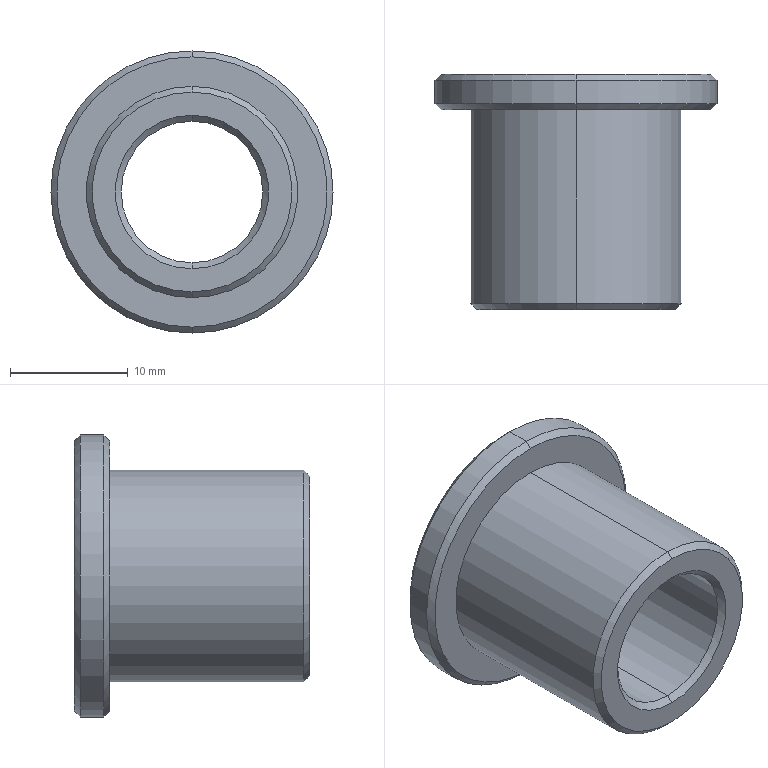Part | SolidWorks | features BaseBody 1 | 1 solid | 19 faces | box 24 x 20 x 24 mm | volume 3357 mm3 | cone 10 | cylinder 6 | plane 3 | commonest cylinder face diameters 12.05 x2 17.98 x2 24 x2
STEP:
#1=CARTESIAN_POINT('',(375.1,-76.45,75.025));
#2=VERTEX_POINT('',#1);
#3=CARTESIAN_POINT('',(375.1,-76.45,62.975));
#4=VERTEX_POINT('',#3);
#5=CARTESIAN_POINT('',(375.1,-76.45,69.));
#6=DIRECTION('',(0.,-1.,0.));
#7=DIRECTION('',(0.,0.,1.));
#8=AXIS2_PLACEMENT_3D('',#5,#6,#7);
#9=CIRCLE('',#8,6.025);
#10=EDGE_CURVE('',#2,#4,#9,.T.);
#11=ORIENTED_EDGE('',*,*,#10,.T.);
#12=CARTESIAN_POINT('',(375.1,-75.95,62.475));
#13=VERTEX_POINT('',#12);
#14=CARTESIAN_POINT('',(375.1,-76.2,62.725));
#15=DIRECTION('',(0.,0.7071,-0.7071));
#16=VECTOR('',#15,1000.);
#17=LINE('',#14,#16);
#18=EDGE_CURVE('',#4,#13,#17,.T.);
#19=ORIENTED_EDGE('',*,*,#18,.T.);
#20=CARTESIAN_POINT('',(375.1,-75.95,75.525));
#21=VERTEX_POINT('',#20);
#22=CARTESIAN_POINT('',(375.1,-75.95,69.));
#23=DIRECTION('',(0.,-1.,0.));
#24=DIRECTION('',(0.,0.,1.));
#25=AXIS2_PLACEMENT_3D('',#22,#23,#24);
#26=CIRCLE('',#25,6.525);
#27=EDGE_CURVE('',#21,#13,#26,.T.);
#28=ORIENTED_EDGE('',*,*,#27,.F.);
#29=CARTESIAN_POINT('',(375.1,-76.2,75.275));
#30=DIRECTION('',(0.,0.7071,0.7071));
#31=VECTOR('',#30,1000.);
#32=LINE('',#29,#31);
#33=EDGE_CURVE('',#2,#21,#32,.T.);
#34=ORIENTED_EDGE('',*,*,#33,.F.);
#35=EDGE_LOOP('',(#11,#19,#28,#34));
#36=FACE_OUTER_BOUND('',#35,.T.);
#37=CARTESIAN_POINT('',(375.1,-76.2,69.));
#38=DIRECTION('',(0.,1.,0.));
#39=DIRECTION('',(0.,0.,1.));
#40=AXIS2_PLACEMENT_3D('',#37,#38,#39);
#41=CONICAL_SURFACE('',#40,6.275,0.7854);
#42=ADVANCED_FACE('',(#36),#41,.F.);
#43=CARTESIAN_POINT('',(375.1,-95.45,62.975));
#44=VERTEX_POINT('',#43);
#45=CARTESIAN_POINT('',(375.1,-95.45,75.025));
#46=VERTEX_POINT('',#45);
#47=CARTESIAN_POINT('',(375.1,-95.45,69.));
#48=DIRECTION('',(0.,1.,0.));
#49=DIRECTION('',(0.,0.,-1.));
#50=AXIS2_PLACEMENT_3D('',#47,#48,#49);
#51=CIRCLE('',#50,6.025);
#52=EDGE_CURVE('',#44,#46,#51,.T.);
#53=ORIENTED_EDGE('',*,*,#52,.F.);
#54=CARTESIAN_POINT('',(375.1,-78.95,62.975));
#55=DIRECTION('',(0.,1.,0.));
#56=VECTOR('',#55,1000.);
#57=LINE('',#54,#56);
#58=EDGE_CURVE('',#44,#4,#57,.T.);
#59=ORIENTED_EDGE('',*,*,#58,.T.);
#60=ORIENTED_EDGE('',*,*,#10,.F.);
#61=CARTESIAN_POINT('',(375.1,-78.95,75.025));
#62=DIRECTION('',(0.,1.,0.));
#63=VECTOR('',#62,1000.);
#64=LINE('',#61,#63);
#65=EDGE_CURVE('',#46,#2,#64,.T.);
#66=ORIENTED_EDGE('',*,*,#65,.F.);
#67=EDGE_LOOP('',(#53,#59,#60,#66));
#68=FACE_OUTER_BOUND('',#67,.T.);
#69=CARTESIAN_POINT('',(375.1,-78.95,69.));
#70=DIRECTION('',(0.,1.,0.));
#71=DIRECTION('',(0.,0.,1.));
#72=AXIS2_PLACEMENT_3D('',#69,#70,#71);
#73=CYLINDRICAL_SURFACE('',#72,6.025);
#74=ADVANCED_FACE('',(#68),#73,.F.);
#75=ORIENTED_EDGE('',*,*,#52,.T.);
#76=CARTESIAN_POINT('',(375.1,-95.95,75.525));
#77=VERTEX_POINT('',#76);
#78=CARTESIAN_POINT('',(375.1,-95.7,75.275));
#79=DIRECTION('',(0.,-0.7071,0.7071));
#80=VECTOR('',#79,1000.);
#81=LINE('',#78,#80);
#82=EDGE_CURVE('',#46,#77,#81,.T.);
#83=ORIENTED_EDGE('',*,*,#82,.T.);
#84=CARTESIAN_POINT('',(375.1,-95.95,62.475));
#85=VERTEX_POINT('',#84);
#86=CARTESIAN_POINT('',(375.1,-95.95,69.));
#87=DIRECTION('',(0.,1.,0.));
#88=DIRECTION('',(0.,0.,-1.));
#89=AXIS2_PLACEMENT_3D('',#86,#87,#88);
#90=CIRCLE('',#89,6.525);
#91=EDGE_CURVE('',#85,#77,#90,.T.);
#92=ORIENTED_EDGE('',*,*,#91,.F.);
#93=CARTESIAN_POINT('',(375.1,-95.7,62.725));
#94=DIRECTION('',(0.,-0.7071,-0.7071));
#95=VECTOR('',#94,1000.);
#96=LINE('',#93,#95);
#97=EDGE_CURVE('',#44,#85,#96,.T.);
#98=ORIENTED_EDGE('',*,*,#97,.F.);
#99=EDGE_LOOP('',(#75,#83,#92,#98));
#100=FACE_OUTER_BOUND('',#99,.T.);
#101=CARTESIAN_POINT('',(375.1,-95.7,69.));
#102=DIRECTION('',(0.,-1.,0.));
#103=DIRECTION('',(0.,0.,-1.));
#104=AXIS2_PLACEMENT_3D('',#101,#102,#103);
#105=CONICAL_SURFACE('',#104,6.275,0.7854);
#106=ADVANCED_FACE('',(#100),#105,.F.);
#107=CARTESIAN_POINT('',(375.1,-75.95,80.5));
#108=VERTEX_POINT('',#107);
#109=CARTESIAN_POINT('',(375.1,-75.95,57.5));
#110=VERTEX_POINT('',#109);
#111=CARTESIAN_POINT('',(375.1,-75.95,69.));
#112=DIRECTION('',(0.,1.,0.));
#113=DIRECTION('',(0.,0.,-1.));
#114=AXIS2_PLACEMENT_3D('',#111,#112,#113);
#115=CIRCLE('',#114,11.5);
#116=EDGE_CURVE('',#108,#110,#115,.T.);
#117=ORIENTED_EDGE('',*,*,#116,.F.);
#118=CARTESIAN_POINT('',(375.1,-76.45,81.));
#119=VERTEX_POINT('',#118);
#120=CARTESIAN_POINT('',(375.1,-76.2,80.75));
#121=DIRECTION('',(0.,-0.7071,0.7071));
#122=VECTOR('',#121,1000.);
#123=LINE('',#120,#122);
#124=EDGE_CURVE('',#108,#119,#123,.T.);
#125=ORIENTED_EDGE('',*,*,#124,.T.);
#126=CARTESIAN_POINT('',(375.1,-76.45,57.));
#127=VERTEX_POINT('',#126);
#128=CARTESIAN_POINT('',(375.1,-76.45,69.));
#129=DIRECTION('',(0.,1.,0.));
#130=DIRECTION('',(0.,0.,-1.));
#131=AXIS2_PLACEMENT_3D('',#128,#129,#130);
#132=CIRCLE('',#131,12.);
#133=EDGE_CURVE('',#119,#127,#132,.T.);
#134=ORIENTED_EDGE('',*,*,#133,.T.);
#135=CARTESIAN_POINT('',(375.1,-76.2,57.25));
#136=DIRECTION('',(0.,-0.7071,-0.7071));
#137=VECTOR('',#136,1000.);
#138=LINE('',#135,#137);
#139=EDGE_CURVE('',#110,#127,#138,.T.);
#140=ORIENTED_EDGE('',*,*,#139,.F.);
#141=EDGE_LOOP('',(#117,#125,#134,#140));
#142=FACE_OUTER_BOUND('',#141,.T.);
#143=CARTESIAN_POINT('',(375.1,-76.2,69.));
#144=DIRECTION('',(0.,-1.,0.));
#145=DIRECTION('',(0.,0.,-1.));
#146=AXIS2_PLACEMENT_3D('',#143,#144,#145);
#147=CONICAL_SURFACE('',#146,11.75,0.7854);
#148=ADVANCED_FACE('',(#142),#147,.T.);
#149=CARTESIAN_POINT('',(375.1,-78.45,57.));
#150=VERTEX_POINT('',#149);
#151=CARTESIAN_POINT('',(375.1,-78.45,81.));
#152=VERTEX_POINT('',#151);
#153=CARTESIAN_POINT('',(375.1,-78.45,69.));
#154=DIRECTION('',(0.,-1.,0.));
#155=DIRECTION('',(0.,0.,-1.));
#156=AXIS2_PLACEMENT_3D('',#153,#154,#155);
#157=CIRCLE('',#156,12.);
#158=EDGE_CURVE('',#150,#152,#157,.T.);
#159=ORIENTED_EDGE('',*,*,#158,.F.);
#160=CARTESIAN_POINT('',(375.1,-78.95,57.));
#161=DIRECTION('',(0.,1.,0.));
#162=VECTOR('',#161,1000.);
#163=LINE('',#160,#162);
#164=EDGE_CURVE('',#150,#127,#163,.T.);
#165=ORIENTED_EDGE('',*,*,#164,.T.);
#166=ORIENTED_EDGE('',*,*,#133,.F.);
#167=CARTESIAN_POINT('',(375.1,-78.95,81.));
#168=DIRECTION('',(0.,1.,0.));
#169=VECTOR('',#168,1000.);
#170=LINE('',#167,#169);
#171=EDGE_CURVE('',#152,#119,#170,.T.);
#172=ORIENTED_EDGE('',*,*,#171,.F.);
#173=EDGE_LOOP('',(#159,#165,#166,#172));
#174=FACE_OUTER_BOUND('',#173,.T.);
#175=CARTESIAN_POINT('',(375.1,-78.95,69.));
#176=DIRECTION('',(0.,1.,0.));
#177=DIRECTION('',(0.,0.,1.));
#178=AXIS2_PLACEMENT_3D('',#175,#176,#177);
#179=CYLINDRICAL_SURFACE('',#178,12.);
#180=ADVANCED_FACE('',(#174),#179,.T.);
#181=CARTESIAN_POINT('',(375.1,-78.95,57.5));
#182=VERTEX_POINT('',#181);
#183=CARTESIAN_POINT('',(375.1,-78.95,80.5));
#184=VERTEX_POINT('',#183);
#185=CARTESIAN_POINT('',(375.1,-78.95,69.));
#186=DIRECTION('',(0.,-1.,0.));
#187=DIRECTION('',(0.,0.,1.));
#188=AXIS2_PLACEMENT_3D('',#185,#186,#187);
#189=CIRCLE('',#188,11.5);
#190=EDGE_CURVE('',#182,#184,#189,.T.);
#191=ORIENTED_EDGE('',*,*,#190,.F.);
#192=CARTESIAN_POINT('',(375.1,-78.7,57.25));
#193=DIRECTION('',(0.,0.7071,-0.7071));
#194=VECTOR('',#193,1000.);
#195=LINE('',#192,#194);
#196=EDGE_CURVE('',#182,#150,#195,.T.);
#197=ORIENTED_EDGE('',*,*,#196,.T.);
#198=ORIENTED_EDGE('',*,*,#158,.T.);
#199=CARTESIAN_POINT('',(375.1,-78.7,80.75));
#200=DIRECTION('',(0.,0.7071,0.7071));
#201=VECTOR('',#200,1000.);
#202=LINE('',#199,#201);
#203=EDGE_CURVE('',#184,#152,#202,.T.);
#204=ORIENTED_EDGE('',*,*,#203,.F.);
#205=EDGE_LOOP('',(#191,#197,#198,#204));
#206=FACE_OUTER_BOUND('',#205,.T.);
#207=CARTESIAN_POINT('',(375.1,-78.7,69.));
#208=DIRECTION('',(0.,1.,0.));
#209=DIRECTION('',(0.,0.,1.));
#210=AXIS2_PLACEMENT_3D('',#207,#208,#209);
#211=CONICAL_SURFACE('',#210,11.75,0.7854);
#212=ADVANCED_FACE('',(#206),#211,.T.);
#213=CARTESIAN_POINT('',(375.1,-95.45,60.01));
#214=VERTEX_POINT('',#213);
#215=CARTESIAN_POINT('',(375.1,-95.45,77.99));
#216=VERTEX_POINT('',#215);
#217=CARTESIAN_POINT('',(375.1,-95.45,69.));
#218=DIRECTION('',(0.,-1.,0.));
#219=DIRECTION('',(0.,0.,-1.));
#220=AXIS2_PLACEMENT_3D('',#217,#218,#219);
#221=CIRCLE('',#220,8.99);
#222=EDGE_CURVE('',#214,#216,#221,.T.);
#223=ORIENTED_EDGE('',*,*,#222,.F.);
#224=CARTESIAN_POINT('',(375.1,-78.95,60.01));
#225=VERTEX_POINT('',#224);
#226=CARTESIAN_POINT('',(375.1,-95.95,60.01));
#227=DIRECTION('',(0.,1.,0.));
#228=VECTOR('',#227,1000.);
#229=LINE('',#226,#228);
#230=EDGE_CURVE('',#214,#225,#229,.T.);
#231=ORIENTED_EDGE('',*,*,#230,.T.);
#232=CARTESIAN_POINT('',(375.1,-78.95,77.99));
#233=VERTEX_POINT('',#232);
#234=CARTESIAN_POINT('',(375.1,-78.95,69.));
#235=DIRECTION('',(0.,1.,0.));
#236=DIRECTION('',(0.,0.,-1.));
#237=AXIS2_PLACEMENT_3D('',#234,#235,#236);
#238=CIRCLE('',#237,8.99);
#239=EDGE_CURVE('',#233,#225,#238,.T.);
#240=ORIENTED_EDGE('',*,*,#239,.F.);
#241=CARTESIAN_POINT('',(375.1,-95.95,77.99));
#242=DIRECTION('',(0.,1.,0.));
#243=VECTOR('',#242,1000.);
#244=LINE('',#241,#243);
#245=EDGE_CURVE('',#216,#233,#244,.T.);
#246=ORIENTED_EDGE('',*,*,#245,.F.);
#247=EDGE_LOOP('',(#223,#231,#240,#246));
#248=FACE_OUTER_BOUND('',#247,.T.);
#249=CARTESIAN_POINT('',(375.1,-95.95,69.));
#250=DIRECTION('',(0.,1.,0.));
#251=DIRECTION('',(0.,0.,1.));
#252=AXIS2_PLACEMENT_3D('',#249,#250,#251);
#253=CYLINDRICAL_SURFACE('',#252,8.99);
#254=ADVANCED_FACE('',(#248),#253,.T.);
#255=CARTESIAN_POINT('',(375.1,-95.95,60.51));
#256=VERTEX_POINT('',#255);
#257=CARTESIAN_POINT('',(375.1,-95.95,77.49));
#258=VERTEX_POINT('',#257);
#259=CARTESIAN_POINT('',(375.1,-95.95,69.));
#260=DIRECTION('',(0.,-1.,0.));
#261=DIRECTION('',(0.,0.,-1.));
#262=AXIS2_PLACEMENT_3D('',#259,#260,#261);
#263=CIRCLE('',#262,8.49);
#264=EDGE_CURVE('',#256,#258,#263,.T.);
#265=ORIENTED_EDGE('',*,*,#264,.F.);
#266=CARTESIAN_POINT('',(375.1,-95.7,60.26));
#267=DIRECTION('',(0.,0.7071,-0.7071));
#268=VECTOR('',#267,1000.);
#269=LINE('',#266,#268);
#270=EDGE_CURVE('',#256,#214,#269,.T.);
#271=ORIENTED_EDGE('',*,*,#270,.T.);
#272=ORIENTED_EDGE('',*,*,#222,.T.);
#273=CARTESIAN_POINT('',(375.1,-95.7,77.74));
#274=DIRECTION('',(0.,0.7071,0.7071));
#275=VECTOR('',#274,1000.);
#276=LINE('',#273,#275);
#277=EDGE_CURVE('',#258,#216,#276,.T.);
#278=ORIENTED_EDGE('',*,*,#277,.F.);
#279=EDGE_LOOP('',(#265,#271,#272,#278));
#280=FACE_OUTER_BOUND('',#279,.T.);
#281=CARTESIAN_POINT('',(375.1,-95.7,69.));
#282=DIRECTION('',(0.,1.,0.));
#283=DIRECTION('',(0.,0.,1.));
#284=AXIS2_PLACEMENT_3D('',#281,#282,#283);
#285=CONICAL_SURFACE('',#284,8.74,0.7854);
#286=ADVANCED_FACE('',(#280),#285,.T.);
#287=ORIENTED_EDGE('',*,*,#91,.T.);
#288=CARTESIAN_POINT('',(375.1,-95.95,69.));
#289=DIRECTION('',(0.,1.,0.));
#290=DIRECTION('',(0.,0.,-1.));
#291=AXIS2_PLACEMENT_3D('',#288,#289,#290);
#292=CIRCLE('',#291,6.525);
#293=EDGE_CURVE('',#77,#85,#292,.T.);
#294=ORIENTED_EDGE('',*,*,#293,.T.);
#295=EDGE_LOOP('',(#287,#294));
#296=FACE_BOUND('',#295,.T.);
#297=CARTESIAN_POINT('',(375.1,-95.95,69.));
#298=DIRECTION('',(0.,-1.,0.));
#299=DIRECTION('',(0.,0.,-1.));
#300=AXIS2_PLACEMENT_3D('',#297,#298,#299);
#301=CIRCLE('',#300,8.49);
#302=EDGE_CURVE('',#258,#256,#301,.T.);
#303=ORIENTED_EDGE('',*,*,#302,.T.);
#304=ORIENTED_EDGE('',*,*,#264,.T.);
#305=EDGE_LOOP('',(#303,#304));
#306=FACE_OUTER_BOUND('',#305,.T.);
#307=CARTESIAN_POINT('',(375.1,-95.95,69.));
#308=DIRECTION('',(0.,-1.,0.));
#309=DIRECTION('',(0.,0.,-1.));
#310=AXIS2_PLACEMENT_3D('',#307,#308,#309);
#311=PLANE('',#310);
#312=ADVANCED_FACE('',(#296,#306),#311,.T.);
#313=ORIENTED_EDGE('',*,*,#270,.F.);
#314=ORIENTED_EDGE('',*,*,#302,.F.);
#315=ORIENTED_EDGE('',*,*,#277,.T.);
#316=CARTESIAN_POINT('',(375.1,-95.45,69.));
#317=DIRECTION('',(0.,-1.,0.));
#318=DIRECTION('',(0.,0.,-1.));
#319=AXIS2_PLACEMENT_3D('',#316,#317,#318);
#320=CIRCLE('',#319,8.99);
#321=EDGE_CURVE('',#216,#214,#320,.T.);
#322=ORIENTED_EDGE('',*,*,#321,.T.);
#323=EDGE_LOOP('',(#313,#314,#315,#322));
#324=FACE_OUTER_BOUND('',#323,.T.);
#325=CARTESIAN_POINT('',(375.1,-95.7,69.));
#326=DIRECTION('',(0.,1.,0.));
#327=DIRECTION('',(0.,0.,1.));
#328=AXIS2_PLACEMENT_3D('',#325,#326,#327);
#329=CONICAL_SURFACE('',#328,8.74,0.7854);
#330=ADVANCED_FACE('',(#324),#329,.T.);
#331=ORIENTED_EDGE('',*,*,#230,.F.);
#332=ORIENTED_EDGE('',*,*,#321,.F.);
#333=ORIENTED_EDGE('',*,*,#245,.T.);
#334=CARTESIAN_POINT('',(375.1,-78.95,69.));
#335=DIRECTION('',(0.,1.,0.));
#336=DIRECTION('',(0.,0.,-1.));
#337=AXIS2_PLACEMENT_3D('',#334,#335,#336);
#338=CIRCLE('',#337,8.99);
#339=EDGE_CURVE('',#225,#233,#338,.T.);
#340=ORIENTED_EDGE('',*,*,#339,.F.);
#341=EDGE_LOOP('',(#331,#332,#333,#340));
#342=FACE_OUTER_BOUND('',#341,.T.);
#343=CARTESIAN_POINT('',(375.1,-95.95,69.));
#344=DIRECTION('',(0.,1.,0.));
#345=DIRECTION('',(0.,0.,1.));
#346=AXIS2_PLACEMENT_3D('',#343,#344,#345);
#347=CYLINDRICAL_SURFACE('',#346,8.99);
#348=ADVANCED_FACE('',(#342),#347,.T.);
#349=ORIENTED_EDGE('',*,*,#239,.T.);
#350=ORIENTED_EDGE('',*,*,#339,.T.);
#351=EDGE_LOOP('',(#349,#350));
#352=FACE_BOUND('',#351,.T.);
#353=CARTESIAN_POINT('',(375.1,-78.95,69.));
#354=DIRECTION('',(0.,-1.,0.));
#355=DIRECTION('',(0.,0.,1.));
#356=AXIS2_PLACEMENT_3D('',#353,#354,#355);
#357=CIRCLE('',#356,11.5);
#358=EDGE_CURVE('',#184,#182,#357,.T.);
#359=ORIENTED_EDGE('',*,*,#358,.T.);
#360=ORIENTED_EDGE('',*,*,#190,.T.);
#361=EDGE_LOOP('',(#359,#360));
#362=FACE_OUTER_BOUND('',#361,.T.);
#363=CARTESIAN_POINT('',(375.1,-78.95,69.));
#364=DIRECTION('',(0.,-1.,0.));
#365=DIRECTION('',(0.,0.,-1.));
#366=AXIS2_PLACEMENT_3D('',#363,#364,#365);
#367=PLANE('',#366);
#368=ADVANCED_FACE('',(#352,#362),#367,.T.);
#369=ORIENTED_EDGE('',*,*,#196,.F.);
#370=ORIENTED_EDGE('',*,*,#358,.F.);
#371=ORIENTED_EDGE('',*,*,#203,.T.);
#372=CARTESIAN_POINT('',(375.1,-78.45,69.));
#373=DIRECTION('',(0.,-1.,0.));
#374=DIRECTION('',(0.,0.,-1.));
#375=AXIS2_PLACEMENT_3D('',#372,#373,#374);
#376=CIRCLE('',#375,12.);
#377=EDGE_CURVE('',#152,#150,#376,.T.);
#378=ORIENTED_EDGE('',*,*,#377,.T.);
#379=EDGE_LOOP('',(#369,#370,#371,#378));
#380=FACE_OUTER_BOUND('',#379,.T.);
#381=CARTESIAN_POINT('',(375.1,-78.7,69.));
#382=DIRECTION('',(0.,1.,0.));
#383=DIRECTION('',(0.,0.,1.));
#384=AXIS2_PLACEMENT_3D('',#381,#382,#383);
#385=CONICAL_SURFACE('',#384,11.75,0.7854);
#386=ADVANCED_FACE('',(#380),#385,.T.);
#387=ORIENTED_EDGE('',*,*,#164,.F.);
#388=ORIENTED_EDGE('',*,*,#377,.F.);
#389=ORIENTED_EDGE('',*,*,#171,.T.);
#390=CARTESIAN_POINT('',(375.1,-76.45,69.));
#391=DIRECTION('',(0.,1.,0.));
#392=DIRECTION('',(0.,0.,-1.));
#393=AXIS2_PLACEMENT_3D('',#390,#391,#392);
#394=CIRCLE('',#393,12.);
#395=EDGE_CURVE('',#127,#119,#394,.T.);
#396=ORIENTED_EDGE('',*,*,#395,.F.);
#397=EDGE_LOOP('',(#387,#388,#389,#396));
#398=FACE_OUTER_BOUND('',#397,.T.);
#399=CARTESIAN_POINT('',(375.1,-78.95,69.));
#400=DIRECTION('',(0.,1.,0.));
#401=DIRECTION('',(0.,0.,1.));
#402=AXIS2_PLACEMENT_3D('',#399,#400,#401);
#403=CYLINDRICAL_SURFACE('',#402,12.);
#404=ADVANCED_FACE('',(#398),#403,.T.);
#405=ORIENTED_EDGE('',*,*,#124,.F.);
#406=CARTESIAN_POINT('',(375.1,-75.95,69.));
#407=DIRECTION('',(0.,1.,0.));
#408=DIRECTION('',(0.,0.,-1.));
#409=AXIS2_PLACEMENT_3D('',#406,#407,#408);
#410=CIRCLE('',#409,11.5);
#411=EDGE_CURVE('',#110,#108,#410,.T.);
#412=ORIENTED_EDGE('',*,*,#411,.F.);
#413=ORIENTED_EDGE('',*,*,#139,.T.);
#414=ORIENTED_EDGE('',*,*,#395,.T.);
#415=EDGE_LOOP('',(#405,#412,#413,#414));
#416=FACE_OUTER_BOUND('',#415,.T.);
#417=CARTESIAN_POINT('',(375.1,-76.2,69.));
#418=DIRECTION('',(0.,-1.,0.));
#419=DIRECTION('',(0.,0.,-1.));
#420=AXIS2_PLACEMENT_3D('',#417,#418,#419);
#421=CONICAL_SURFACE('',#420,11.75,0.7854);
#422=ADVANCED_FACE('',(#416),#421,.T.);
#423=ORIENTED_EDGE('',*,*,#27,.T.);
#424=CARTESIAN_POINT('',(375.1,-75.95,69.));
#425=DIRECTION('',(0.,-1.,0.));
#426=DIRECTION('',(0.,0.,1.));
#427=AXIS2_PLACEMENT_3D('',#424,#425,#426);
#428=CIRCLE('',#427,6.525);
#429=EDGE_CURVE('',#13,#21,#428,.T.);
#430=ORIENTED_EDGE('',*,*,#429,.T.);
#431=EDGE_LOOP('',(#423,#430));
#432=FACE_BOUND('',#431,.T.);
#433=ORIENTED_EDGE('',*,*,#411,.T.);
#434=ORIENTED_EDGE('',*,*,#116,.T.);
#435=EDGE_LOOP('',(#433,#434));
#436=FACE_OUTER_BOUND('',#435,.T.);
#437=CARTESIAN_POINT('',(375.1,-75.95,69.));
#438=DIRECTION('',(0.,-1.,0.));
#439=DIRECTION('',(0.,0.,-1.));
#440=AXIS2_PLACEMENT_3D('',#437,#438,#439);
#441=PLANE('',#440);
#442=ADVANCED_FACE('',(#432,#436),#441,.F.);
#443=ORIENTED_EDGE('',*,*,#82,.F.);
#444=CARTESIAN_POINT('',(375.1,-95.45,69.));
#445=DIRECTION('',(0.,1.,0.));
#446=DIRECTION('',(0.,0.,-1.));
#447=AXIS2_PLACEMENT_3D('',#444,#445,#446);
#448=CIRCLE('',#447,6.025);
#449=EDGE_CURVE('',#46,#44,#448,.T.);
#450=ORIENTED_EDGE('',*,*,#449,.T.);
#451=ORIENTED_EDGE('',*,*,#97,.T.);
#452=ORIENTED_EDGE('',*,*,#293,.F.);
#453=EDGE_LOOP('',(#443,#450,#451,#452));
#454=FACE_OUTER_BOUND('',#453,.T.);
#455=CARTESIAN_POINT('',(375.1,-95.7,69.));
#456=DIRECTION('',(0.,-1.,0.));
#457=DIRECTION('',(0.,0.,-1.));
#458=AXIS2_PLACEMENT_3D('',#455,#456,#457);
#459=CONICAL_SURFACE('',#458,6.275,0.7854);
#460=ADVANCED_FACE('',(#454),#459,.F.);
#461=ORIENTED_EDGE('',*,*,#58,.F.);
#462=ORIENTED_EDGE('',*,*,#449,.F.);
#463=ORIENTED_EDGE('',*,*,#65,.T.);
#464=CARTESIAN_POINT('',(375.1,-76.45,69.));
#465=DIRECTION('',(0.,-1.,0.));
#466=DIRECTION('',(0.,0.,1.));
#467=AXIS2_PLACEMENT_3D('',#464,#465,#466);
#468=CIRCLE('',#467,6.025);
#469=EDGE_CURVE('',#4,#2,#468,.T.);
#470=ORIENTED_EDGE('',*,*,#469,.F.);
#471=EDGE_LOOP('',(#461,#462,#463,#470));
#472=FACE_OUTER_BOUND('',#471,.T.);
#473=CARTESIAN_POINT('',(375.1,-78.95,69.));
#474=DIRECTION('',(0.,1.,0.));
#475=DIRECTION('',(0.,0.,1.));
#476=AXIS2_PLACEMENT_3D('',#473,#474,#475);
#477=CYLINDRICAL_SURFACE('',#476,6.025);
#478=ADVANCED_FACE('',(#472),#477,.F.);
#479=ORIENTED_EDGE('',*,*,#18,.F.);
#480=ORIENTED_EDGE('',*,*,#469,.T.);
#481=ORIENTED_EDGE('',*,*,#33,.T.);
#482=ORIENTED_EDGE('',*,*,#429,.F.);
#483=EDGE_LOOP('',(#479,#480,#481,#482));
#484=FACE_OUTER_BOUND('',#483,.T.);
#485=CARTESIAN_POINT('',(375.1,-76.2,69.));
#486=DIRECTION('',(0.,1.,0.));
#487=DIRECTION('',(0.,0.,1.));
#488=AXIS2_PLACEMENT_3D('',#485,#486,#487);
#489=CONICAL_SURFACE('',#488,6.275,0.7854);
#490=ADVANCED_FACE('',(#484),#489,.F.);
#491=CLOSED_SHELL('',(#42,#74,#106,#148,#180,#212,#254,#286,#312,#330,#348,#368,#386,#404,#422,#442,#460,#478,#490));
#492=MANIFOLD_SOLID_BREP('',#491);
#493=CARTESIAN_POINT('',(0.,0.,0.));
#494=DIRECTION('',(0.,0.,1.));
#495=DIRECTION('',(1.,0.,0.));
#496=AXIS2_PLACEMENT_3D('',#493,#494,#495);
#497=(LENGTH_UNIT()NAMED_UNIT(*)SI_UNIT(.MILLI.,.METRE.));
#498=UNCERTAINTY_MEASURE_WITH_UNIT(LENGTH_MEASURE(0.00001),#497,'','');
#499=(NAMED_UNIT(*)PLANE_ANGLE_UNIT()SI_UNIT($,.RADIAN.));
#500=(NAMED_UNIT(*)SI_UNIT($,.STERADIAN.)SOLID_ANGLE_UNIT());
#501=(GEOMETRIC_REPRESENTATION_CONTEXT(3)GLOBAL_UNCERTAINTY_ASSIGNED_CONTEXT((#498))GLOBAL_UNIT_ASSIGNED_CONTEXT((#497,#499,#500))REPRESENTATION_CONTEXT('',''));
#502=ADVANCED_BREP_SHAPE_REPRESENTATION('',(#492,#496),#501);